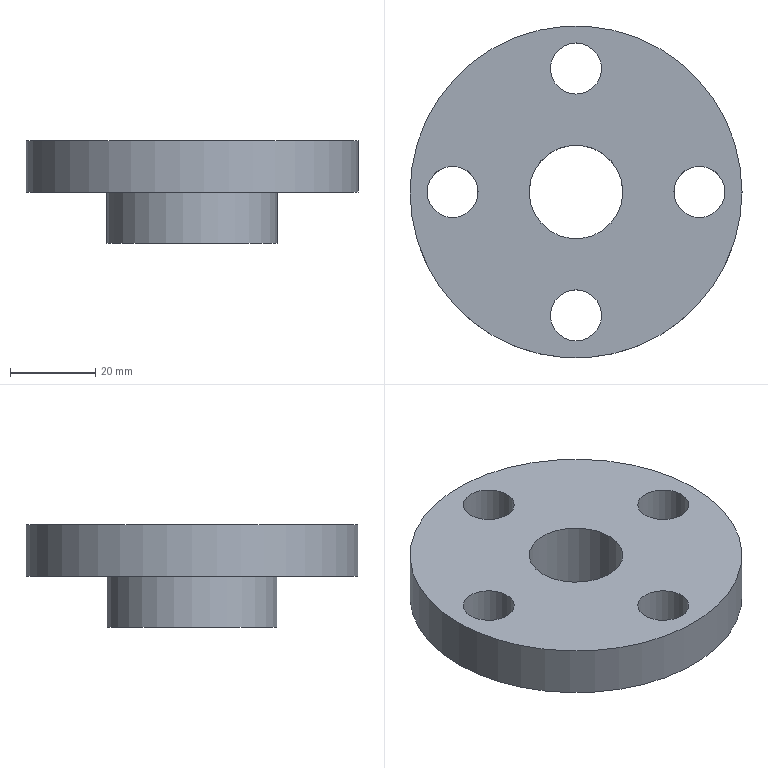Part | NX | 1 solid | 10 faces | box 78 x 78 x 24 mm | volume 57868 mm3 | cylinder 7 | plane 3 | commonest cylinder face diameters 12 x4 22 x1 40 x1 78 x1
STEP:
#1=CARTESIAN_POINT('',(-20.,0.,-12.));
#2=VERTEX_POINT('',#1);
#3=CARTESIAN_POINT('',(0.,0.,-12.));
#4=DIRECTION('',(0.,0.,-1.));
#5=DIRECTION('',(-1.,0.,0.));
#6=AXIS2_PLACEMENT_3D('',#3,#4,#5);
#7=CIRCLE('',#6,20.);
#8=EDGE_CURVE('',#2,#2,#7,.F.);
#9=ORIENTED_EDGE('',*,*,#8,.F.);
#10=EDGE_LOOP('',(#9));
#11=FACE_BOUND('',#10,.T.);
#12=CARTESIAN_POINT('',(20.,0.,-24.));
#13=VERTEX_POINT('',#12);
#14=CARTESIAN_POINT('',(0.,0.,-24.));
#15=DIRECTION('',(0.,0.,1.));
#16=DIRECTION('',(1.,0.,0.));
#17=AXIS2_PLACEMENT_3D('',#14,#15,#16);
#18=CIRCLE('',#17,20.);
#19=EDGE_CURVE('',#13,#13,#18,.T.);
#20=ORIENTED_EDGE('',*,*,#19,.T.);
#21=EDGE_LOOP('',(#20));
#22=FACE_BOUND('',#21,.T.);
#23=CARTESIAN_POINT('',(0.,0.,-24.));
#24=DIRECTION('',(0.,0.,1.));
#25=DIRECTION('',(1.,0.,0.));
#26=AXIS2_PLACEMENT_3D('',#23,#24,#25);
#27=CYLINDRICAL_SURFACE('',#26,20.);
#28=ADVANCED_FACE('',(#11,#22),#27,.T.);
#29=CARTESIAN_POINT('',(11.,0.,-24.));
#30=VERTEX_POINT('',#29);
#31=CARTESIAN_POINT('',(0.,0.,-24.));
#32=DIRECTION('',(0.,0.,-1.));
#33=DIRECTION('',(1.,0.,0.));
#34=AXIS2_PLACEMENT_3D('',#31,#32,#33);
#35=CIRCLE('',#34,11.);
#36=EDGE_CURVE('',#30,#30,#35,.T.);
#37=ORIENTED_EDGE('',*,*,#36,.T.);
#38=EDGE_LOOP('',(#37));
#39=FACE_BOUND('',#38,.T.);
#40=CARTESIAN_POINT('',(11.,0.,0.));
#41=VERTEX_POINT('',#40);
#42=CARTESIAN_POINT('',(0.,0.,0.));
#43=DIRECTION('',(0.,0.,-1.));
#44=DIRECTION('',(1.,0.,0.));
#45=AXIS2_PLACEMENT_3D('',#42,#43,#44);
#46=CIRCLE('',#45,11.);
#47=EDGE_CURVE('',#41,#41,#46,.T.);
#48=ORIENTED_EDGE('',*,*,#47,.F.);
#49=EDGE_LOOP('',(#48));
#50=FACE_BOUND('',#49,.T.);
#51=CARTESIAN_POINT('',(0.,0.,-24.));
#52=DIRECTION('',(0.,0.,1.));
#53=DIRECTION('',(1.,0.,0.));
#54=AXIS2_PLACEMENT_3D('',#51,#52,#53);
#55=CYLINDRICAL_SURFACE('',#54,11.);
#56=ADVANCED_FACE('',(#39,#50),#55,.F.);
#57=ORIENTED_EDGE('',*,*,#19,.F.);
#58=EDGE_LOOP('',(#57));
#59=FACE_BOUND('',#58,.T.);
#60=ORIENTED_EDGE('',*,*,#36,.F.);
#61=EDGE_LOOP('',(#60));
#62=FACE_BOUND('',#61,.T.);
#63=CARTESIAN_POINT('',(0.,0.,-24.));
#64=DIRECTION('',(0.,0.,1.));
#65=DIRECTION('',(1.,0.,0.));
#66=AXIS2_PLACEMENT_3D('',#63,#64,#65);
#67=PLANE('',#66);
#68=ADVANCED_FACE('',(#59,#62),#67,.F.);
#69=ORIENTED_EDGE('',*,*,#47,.T.);
#70=EDGE_LOOP('',(#69));
#71=FACE_BOUND('',#70,.T.);
#72=CARTESIAN_POINT('',(39.,0.,0.));
#73=VERTEX_POINT('',#72);
#74=CARTESIAN_POINT('',(0.,0.,0.));
#75=DIRECTION('',(0.,0.,-1.));
#76=DIRECTION('',(1.,0.,0.));
#77=AXIS2_PLACEMENT_3D('',#74,#75,#76);
#78=CIRCLE('',#77,39.);
#79=EDGE_CURVE('',#73,#73,#78,.T.);
#80=ORIENTED_EDGE('',*,*,#79,.F.);
#81=EDGE_LOOP('',(#80));
#82=FACE_BOUND('',#81,.T.);
#83=CARTESIAN_POINT('',(35.,0.,0.));
#84=VERTEX_POINT('',#83);
#85=CARTESIAN_POINT('',(29.,0.,0.));
#86=DIRECTION('',(0.,0.,1.));
#87=DIRECTION('',(1.,0.,0.));
#88=AXIS2_PLACEMENT_3D('',#85,#86,#87);
#89=CIRCLE('',#88,6.);
#90=EDGE_CURVE('',#84,#84,#89,.T.);
#91=ORIENTED_EDGE('',*,*,#90,.F.);
#92=EDGE_LOOP('',(#91));
#93=FACE_BOUND('',#92,.T.);
#94=CARTESIAN_POINT('',(0.,35.,0.));
#95=VERTEX_POINT('',#94);
#96=CARTESIAN_POINT('',(0.,29.,0.));
#97=DIRECTION('',(0.,0.,1.));
#98=DIRECTION('',(0.,1.,0.));
#99=AXIS2_PLACEMENT_3D('',#96,#97,#98);
#100=CIRCLE('',#99,6.);
#101=EDGE_CURVE('',#95,#95,#100,.T.);
#102=ORIENTED_EDGE('',*,*,#101,.F.);
#103=EDGE_LOOP('',(#102));
#104=FACE_BOUND('',#103,.T.);
#105=CARTESIAN_POINT('',(0.,-35.,0.));
#106=VERTEX_POINT('',#105);
#107=CARTESIAN_POINT('',(0.,-29.,0.));
#108=DIRECTION('',(0.,0.,1.));
#109=DIRECTION('',(0.,-1.,0.));
#110=AXIS2_PLACEMENT_3D('',#107,#108,#109);
#111=CIRCLE('',#110,6.);
#112=EDGE_CURVE('',#106,#106,#111,.T.);
#113=ORIENTED_EDGE('',*,*,#112,.F.);
#114=EDGE_LOOP('',(#113));
#115=FACE_BOUND('',#114,.T.);
#116=CARTESIAN_POINT('',(-35.,0.,0.));
#117=VERTEX_POINT('',#116);
#118=CARTESIAN_POINT('',(-29.,0.,0.));
#119=DIRECTION('',(0.,0.,1.));
#120=DIRECTION('',(-1.,0.,0.));
#121=AXIS2_PLACEMENT_3D('',#118,#119,#120);
#122=CIRCLE('',#121,6.);
#123=EDGE_CURVE('',#117,#117,#122,.T.);
#124=ORIENTED_EDGE('',*,*,#123,.F.);
#125=EDGE_LOOP('',(#124));
#126=FACE_BOUND('',#125,.T.);
#127=CARTESIAN_POINT('',(0.,0.,0.));
#128=DIRECTION('',(0.,0.,1.));
#129=DIRECTION('',(1.,0.,0.));
#130=AXIS2_PLACEMENT_3D('',#127,#128,#129);
#131=PLANE('',#130);
#132=ADVANCED_FACE('',(#71,#82,#93,#104,#115,#126),#131,.T.);
#133=CARTESIAN_POINT('',(0.,-35.,-12.));
#134=VERTEX_POINT('',#133);
#135=CARTESIAN_POINT('',(0.,-29.,-12.));
#136=DIRECTION('',(0.,0.,1.));
#137=DIRECTION('',(0.,-1.,0.));
#138=AXIS2_PLACEMENT_3D('',#135,#136,#137);
#139=CIRCLE('',#138,6.);
#140=EDGE_CURVE('',#134,#134,#139,.T.);
#141=ORIENTED_EDGE('',*,*,#140,.F.);
#142=EDGE_LOOP('',(#141));
#143=FACE_BOUND('',#142,.T.);
#144=ORIENTED_EDGE('',*,*,#112,.T.);
#145=EDGE_LOOP('',(#144));
#146=FACE_BOUND('',#145,.T.);
#147=CARTESIAN_POINT('',(0.,-29.,-12.));
#148=DIRECTION('',(0.,0.,1.));
#149=DIRECTION('',(1.,0.,0.));
#150=AXIS2_PLACEMENT_3D('',#147,#148,#149);
#151=CYLINDRICAL_SURFACE('',#150,6.);
#152=ADVANCED_FACE('',(#143,#146),#151,.F.);
#153=CARTESIAN_POINT('',(0.,35.,-12.));
#154=VERTEX_POINT('',#153);
#155=CARTESIAN_POINT('',(0.,29.,-12.));
#156=DIRECTION('',(0.,0.,1.));
#157=DIRECTION('',(0.,1.,0.));
#158=AXIS2_PLACEMENT_3D('',#155,#156,#157);
#159=CIRCLE('',#158,6.);
#160=EDGE_CURVE('',#154,#154,#159,.T.);
#161=ORIENTED_EDGE('',*,*,#160,.F.);
#162=EDGE_LOOP('',(#161));
#163=FACE_BOUND('',#162,.T.);
#164=ORIENTED_EDGE('',*,*,#101,.T.);
#165=EDGE_LOOP('',(#164));
#166=FACE_BOUND('',#165,.T.);
#167=CARTESIAN_POINT('',(0.,29.,-12.));
#168=DIRECTION('',(0.,0.,1.));
#169=DIRECTION('',(1.,0.,0.));
#170=AXIS2_PLACEMENT_3D('',#167,#168,#169);
#171=CYLINDRICAL_SURFACE('',#170,6.);
#172=ADVANCED_FACE('',(#163,#166),#171,.F.);
#173=CARTESIAN_POINT('',(35.,0.,-12.));
#174=VERTEX_POINT('',#173);
#175=CARTESIAN_POINT('',(29.,0.,-12.));
#176=DIRECTION('',(0.,0.,1.));
#177=DIRECTION('',(1.,0.,0.));
#178=AXIS2_PLACEMENT_3D('',#175,#176,#177);
#179=CIRCLE('',#178,6.);
#180=EDGE_CURVE('',#174,#174,#179,.T.);
#181=ORIENTED_EDGE('',*,*,#180,.F.);
#182=EDGE_LOOP('',(#181));
#183=FACE_BOUND('',#182,.T.);
#184=ORIENTED_EDGE('',*,*,#90,.T.);
#185=EDGE_LOOP('',(#184));
#186=FACE_BOUND('',#185,.T.);
#187=CARTESIAN_POINT('',(29.,0.,-12.));
#188=DIRECTION('',(0.,0.,1.));
#189=DIRECTION('',(1.,0.,0.));
#190=AXIS2_PLACEMENT_3D('',#187,#188,#189);
#191=CYLINDRICAL_SURFACE('',#190,6.);
#192=ADVANCED_FACE('',(#183,#186),#191,.F.);
#193=CARTESIAN_POINT('',(39.,0.,-12.));
#194=VERTEX_POINT('',#193);
#195=CARTESIAN_POINT('',(0.,0.,-12.));
#196=DIRECTION('',(0.,0.,-1.));
#197=DIRECTION('',(1.,0.,0.));
#198=AXIS2_PLACEMENT_3D('',#195,#196,#197);
#199=CIRCLE('',#198,39.);
#200=EDGE_CURVE('',#194,#194,#199,.T.);
#201=ORIENTED_EDGE('',*,*,#200,.F.);
#202=EDGE_LOOP('',(#201));
#203=FACE_BOUND('',#202,.T.);
#204=ORIENTED_EDGE('',*,*,#79,.T.);
#205=EDGE_LOOP('',(#204));
#206=FACE_BOUND('',#205,.T.);
#207=CARTESIAN_POINT('',(0.,0.,-12.));
#208=DIRECTION('',(0.,0.,1.));
#209=DIRECTION('',(1.,0.,0.));
#210=AXIS2_PLACEMENT_3D('',#207,#208,#209);
#211=CYLINDRICAL_SURFACE('',#210,39.);
#212=ADVANCED_FACE('',(#203,#206),#211,.T.);
#213=CARTESIAN_POINT('',(-35.,0.,-12.));
#214=VERTEX_POINT('',#213);
#215=CARTESIAN_POINT('',(-29.,0.,-12.));
#216=DIRECTION('',(0.,0.,1.));
#217=DIRECTION('',(-1.,0.,0.));
#218=AXIS2_PLACEMENT_3D('',#215,#216,#217);
#219=CIRCLE('',#218,6.);
#220=EDGE_CURVE('',#214,#214,#219,.T.);
#221=ORIENTED_EDGE('',*,*,#220,.F.);
#222=EDGE_LOOP('',(#221));
#223=FACE_BOUND('',#222,.T.);
#224=ORIENTED_EDGE('',*,*,#123,.T.);
#225=EDGE_LOOP('',(#224));
#226=FACE_BOUND('',#225,.T.);
#227=CARTESIAN_POINT('',(-29.,0.,-12.));
#228=DIRECTION('',(0.,0.,1.));
#229=DIRECTION('',(1.,0.,0.));
#230=AXIS2_PLACEMENT_3D('',#227,#228,#229);
#231=CYLINDRICAL_SURFACE('',#230,6.);
#232=ADVANCED_FACE('',(#223,#226),#231,.F.);
#233=ORIENTED_EDGE('',*,*,#200,.T.);
#234=EDGE_LOOP('',(#233));
#235=FACE_BOUND('',#234,.T.);
#236=ORIENTED_EDGE('',*,*,#180,.T.);
#237=EDGE_LOOP('',(#236));
#238=FACE_BOUND('',#237,.T.);
#239=ORIENTED_EDGE('',*,*,#160,.T.);
#240=EDGE_LOOP('',(#239));
#241=FACE_BOUND('',#240,.T.);
#242=ORIENTED_EDGE('',*,*,#140,.T.);
#243=EDGE_LOOP('',(#242));
#244=FACE_BOUND('',#243,.T.);
#245=ORIENTED_EDGE('',*,*,#8,.T.);
#246=EDGE_LOOP('',(#245));
#247=FACE_BOUND('',#246,.T.);
#248=ORIENTED_EDGE('',*,*,#220,.T.);
#249=EDGE_LOOP('',(#248));
#250=FACE_BOUND('',#249,.T.);
#251=CARTESIAN_POINT('',(14.5,0.,-12.));
#252=DIRECTION('',(0.,0.,-1.));
#253=DIRECTION('',(-1.,0.,0.));
#254=AXIS2_PLACEMENT_3D('',#251,#252,#253);
#255=PLANE('',#254);
#256=ADVANCED_FACE('',(#235,#238,#241,#244,#247,#250),#255,.T.);
#257=CLOSED_SHELL('',(#28,#56,#68,#132,#152,#172,#192,#212,#232,#256));
#258=MANIFOLD_SOLID_BREP('',#257);
#259=(LENGTH_UNIT()NAMED_UNIT(*)SI_UNIT(.MILLI.,.METRE.));
#260=UNCERTAINTY_MEASURE_WITH_UNIT(LENGTH_MEASURE(0.00001),#259,'','');
#261=(NAMED_UNIT(*)PLANE_ANGLE_UNIT()SI_UNIT($,.RADIAN.));
#262=(NAMED_UNIT(*)SI_UNIT($,.STERADIAN.)SOLID_ANGLE_UNIT());
#263=(GEOMETRIC_REPRESENTATION_CONTEXT(3)GLOBAL_UNCERTAINTY_ASSIGNED_CONTEXT((#260))GLOBAL_UNIT_ASSIGNED_CONTEXT((#259,#261,#262))REPRESENTATION_CONTEXT('',''));
#264=ADVANCED_BREP_SHAPE_REPRESENTATION('',(#258),#263);